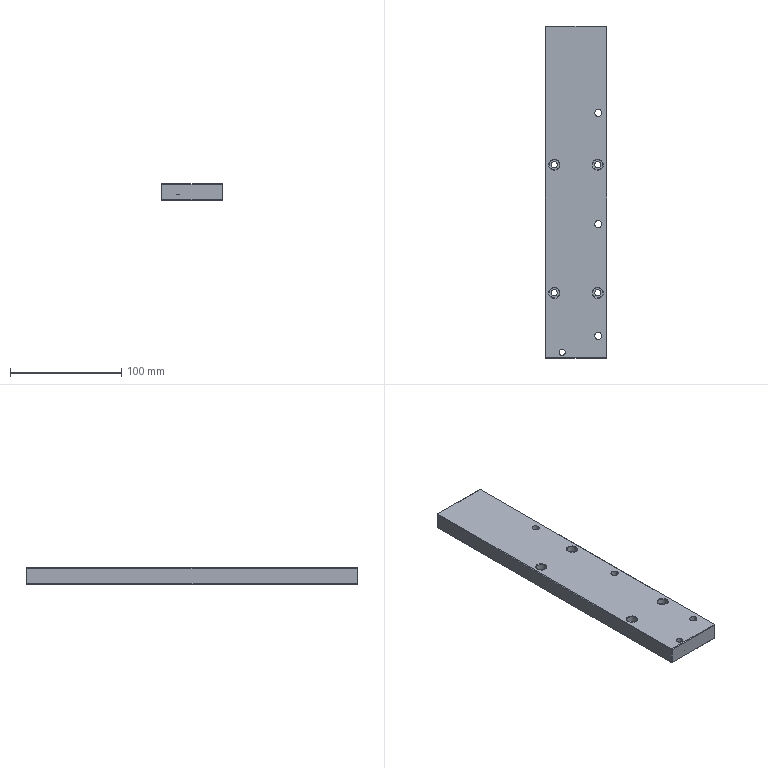Part | 1 solid | 58 faces | box 55 x 298 x 15 mm | volume 240058 mm3 | plane 34 | cylinder 16 | cone 8 | commonest cylinder face diameters 5.5 x5 9 x5 6.5 x3 11 x3
STEP:
#1=CARTESIAN_POINT('',(44.999,-413.,287.5));
#2=VERTEX_POINT('',#1);
#3=CARTESIAN_POINT('',(49.499,-413.,287.5));
#4=DIRECTION('',(0.,0.,-1.));
#5=DIRECTION('',(-1.,0.,0.));
#6=AXIS2_PLACEMENT_3D('',#3,#4,#5);
#7=CIRCLE('',#6,4.5);
#8=EDGE_CURVE('',#2,#2,#7,.T.);
#9=ORIENTED_EDGE('',*,*,#8,.F.);
#10=EDGE_LOOP('',(#9));
#11=FACE_BOUND('',#10,.T.);
#12=CARTESIAN_POINT('',(47.32,-417.5,287.));
#13=VERTEX_POINT('',#12);
#14=CARTESIAN_POINT('',(51.679,-417.5,287.));
#15=VERTEX_POINT('',#14);
#16=CARTESIAN_POINT('',(47.32,-417.5,287.));
#17=CARTESIAN_POINT('',(48.737,-417.825,287.325));
#18=CARTESIAN_POINT('',(50.261,-417.825,287.325));
#19=CARTESIAN_POINT('',(51.679,-417.5,287.));
#20=B_SPLINE_CURVE_WITH_KNOTS('',3,(#16,#17,#18,#19),.UNSPECIFIED.,.F.,.F.,(4,4),(0.,0.004404),.UNSPECIFIED.);
#21=EDGE_CURVE('',#13,#15,#20,.T.);
#22=ORIENTED_EDGE('',*,*,#21,.F.);
#23=CARTESIAN_POINT('',(49.499,-413.,287.));
#24=DIRECTION('',(0.,0.,-1.));
#25=DIRECTION('',(-1.,0.,0.));
#26=AXIS2_PLACEMENT_3D('',#23,#24,#25);
#27=CIRCLE('',#26,5.);
#28=EDGE_CURVE('',#15,#13,#27,.F.);
#29=ORIENTED_EDGE('',*,*,#28,.F.);
#30=EDGE_LOOP('',(#22,#29));
#31=FACE_BOUND('',#30,.T.);
#32=CARTESIAN_POINT('',(49.499,-413.,287.));
#33=DIRECTION('',(0.,0.,-1.));
#34=DIRECTION('',(-1.,0.,0.));
#35=AXIS2_PLACEMENT_3D('',#32,#33,#34);
#36=CONICAL_SURFACE('',#35,5.,0.7854);
#37=ADVANCED_FACE('',(#11,#31),#36,.F.);
#38=CARTESIAN_POINT('',(88.999,-120.,287.5));
#39=VERTEX_POINT('',#38);
#40=CARTESIAN_POINT('',(88.999,-120.5,287.));
#41=VERTEX_POINT('',#40);
#42=CARTESIAN_POINT('',(88.999,-120.5,287.));
#43=DIRECTION('',(0.,-0.7071,-0.7071));
#44=VECTOR('',#43,1000.);
#45=LINE('',#42,#44);
#46=EDGE_CURVE('',#39,#41,#45,.T.);
#47=ORIENTED_EDGE('',*,*,#46,.T.);
#48=CARTESIAN_POINT('',(34.999,-120.5,287.));
#49=VERTEX_POINT('',#48);
#50=CARTESIAN_POINT('',(61.999,-120.5,287.));
#51=DIRECTION('',(1.,0.,0.));
#52=VECTOR('',#51,1000.);
#53=LINE('',#50,#52);
#54=EDGE_CURVE('',#49,#41,#53,.T.);
#55=ORIENTED_EDGE('',*,*,#54,.F.);
#56=CARTESIAN_POINT('',(34.999,-120.,287.5));
#57=VERTEX_POINT('',#56);
#58=CARTESIAN_POINT('',(34.999,-120.,287.5));
#59=DIRECTION('',(0.,0.7071,0.7071));
#60=VECTOR('',#59,1000.);
#61=LINE('',#58,#60);
#62=EDGE_CURVE('',#49,#57,#61,.T.);
#63=ORIENTED_EDGE('',*,*,#62,.T.);
#64=CARTESIAN_POINT('',(38.999,-120.,287.5));
#65=DIRECTION('',(-1.,0.,0.));
#66=VECTOR('',#65,1000.);
#67=LINE('',#64,#66);
#68=EDGE_CURVE('',#39,#57,#67,.T.);
#69=ORIENTED_EDGE('',*,*,#68,.F.);
#70=EDGE_LOOP('',(#47,#55,#63,#69));
#71=FACE_BOUND('',#70,.T.);
#72=CARTESIAN_POINT('',(38.999,-120.,287.5));
#73=DIRECTION('',(0.,0.7071,-0.7071));
#74=DIRECTION('',(1.,0.,0.));
#75=AXIS2_PLACEMENT_3D('',#72,#73,#74);
#76=PLANE('',#75);
#77=ADVANCED_FACE('',(#71),#76,.T.);
#78=CARTESIAN_POINT('',(34.499,-120.5,287.5));
#79=VERTEX_POINT('',#78);
#80=CARTESIAN_POINT('',(34.749,-120.5,287.25));
#81=DIRECTION('',(-0.7071,-0.000000072,0.7071));
#82=VECTOR('',#81,1000.);
#83=LINE('',#80,#82);
#84=EDGE_CURVE('',#49,#79,#83,.T.);
#85=ORIENTED_EDGE('',*,*,#84,.T.);
#86=CARTESIAN_POINT('',(34.999,-120.,287.5));
#87=DIRECTION('',(0.7071,0.7071,0.000000072));
#88=VECTOR('',#87,1000.);
#89=LINE('',#86,#88);
#90=EDGE_CURVE('',#79,#57,#89,.T.);
#91=ORIENTED_EDGE('',*,*,#90,.T.);
#92=ORIENTED_EDGE('',*,*,#62,.F.);
#93=EDGE_LOOP('',(#85,#91,#92));
#94=FACE_BOUND('',#93,.T.);
#95=CARTESIAN_POINT('',(34.999,-120.,287.5));
#96=DIRECTION('',(-0.5774,0.5774,-0.5774));
#97=DIRECTION('',(-0.7071,-0.7071,0.));
#98=AXIS2_PLACEMENT_3D('',#95,#96,#97);
#99=PLANE('',#98);
#100=ADVANCED_FACE('',(#94),#99,.T.);
#101=CARTESIAN_POINT('',(89.499,-120.5,287.5));
#102=VERTEX_POINT('',#101);
#103=CARTESIAN_POINT('',(89.249,-120.25,287.5));
#104=DIRECTION('',(0.7071,-0.7071,-0.000000072));
#105=VECTOR('',#104,1000.);
#106=LINE('',#103,#105);
#107=EDGE_CURVE('',#39,#102,#106,.T.);
#108=ORIENTED_EDGE('',*,*,#107,.T.);
#109=CARTESIAN_POINT('',(88.999,-120.5,287.));
#110=DIRECTION('',(-0.7071,0.000000072,-0.7071));
#111=VECTOR('',#110,1000.);
#112=LINE('',#109,#111);
#113=EDGE_CURVE('',#102,#41,#112,.T.);
#114=ORIENTED_EDGE('',*,*,#113,.T.);
#115=ORIENTED_EDGE('',*,*,#46,.F.);
#116=EDGE_LOOP('',(#108,#114,#115));
#117=FACE_BOUND('',#116,.T.);
#118=CARTESIAN_POINT('',(88.999,-120.5,287.));
#119=DIRECTION('',(0.5774,0.5774,-0.5774));
#120=DIRECTION('',(-0.7071,0.7071,0.));
#121=AXIS2_PLACEMENT_3D('',#118,#119,#120);
#122=PLANE('',#121);
#123=ADVANCED_FACE('',(#117),#122,.T.);
#124=CARTESIAN_POINT('',(34.999,-417.5,287.));
#125=VERTEX_POINT('',#124);
#126=CARTESIAN_POINT('',(34.499,-417.5,287.5));
#127=VERTEX_POINT('',#126);
#128=CARTESIAN_POINT('',(34.499,-417.5,287.5));
#129=DIRECTION('',(-0.7071,-0.000000072,0.7071));
#130=VECTOR('',#129,1000.);
#131=LINE('',#128,#130);
#132=EDGE_CURVE('',#125,#127,#131,.T.);
#133=ORIENTED_EDGE('',*,*,#132,.T.);
#134=CARTESIAN_POINT('',(34.499,-424.5,287.5));
#135=DIRECTION('',(0.,-1.,-0.000000102));
#136=VECTOR('',#135,1000.);
#137=LINE('',#134,#136);
#138=EDGE_CURVE('',#79,#127,#137,.T.);
#139=ORIENTED_EDGE('',*,*,#138,.F.);
#140=ORIENTED_EDGE('',*,*,#84,.F.);
#141=CARTESIAN_POINT('',(34.999,-269.065,287.));
#142=DIRECTION('',(0.000000102,1.,0.));
#143=VECTOR('',#142,1000.);
#144=LINE('',#141,#143);
#145=EDGE_CURVE('',#125,#49,#144,.T.);
#146=ORIENTED_EDGE('',*,*,#145,.F.);
#147=EDGE_LOOP('',(#133,#139,#140,#146));
#148=FACE_BOUND('',#147,.T.);
#149=CARTESIAN_POINT('',(34.499,-424.5,287.5));
#150=DIRECTION('',(-0.7071,0.000000072,-0.7071));
#151=DIRECTION('',(0.,1.,0.000000102));
#152=AXIS2_PLACEMENT_3D('',#149,#150,#151);
#153=PLANE('',#152);
#154=ADVANCED_FACE('',(#148),#153,.T.);
#155=CARTESIAN_POINT('',(34.499,-120.5,301.5));
#156=VERTEX_POINT('',#155);
#157=CARTESIAN_POINT('',(34.999,-120.,301.5));
#158=VERTEX_POINT('',#157);
#159=CARTESIAN_POINT('',(34.499,-120.5,301.5));
#160=DIRECTION('',(0.7071,0.7071,0.000000072));
#161=VECTOR('',#160,1000.);
#162=LINE('',#159,#161);
#163=EDGE_CURVE('',#156,#158,#162,.T.);
#164=ORIENTED_EDGE('',*,*,#163,.T.);
#165=CARTESIAN_POINT('',(34.999,-120.,305.));
#166=DIRECTION('',(0.,-0.000000102,1.));
#167=VECTOR('',#166,1000.);
#168=LINE('',#165,#167);
#169=EDGE_CURVE('',#57,#158,#168,.T.);
#170=ORIENTED_EDGE('',*,*,#169,.F.);
#171=ORIENTED_EDGE('',*,*,#90,.F.);
#172=CARTESIAN_POINT('',(34.499,-120.5,246.881));
#173=DIRECTION('',(0.,0.000000102,-1.));
#174=VECTOR('',#173,1000.);
#175=LINE('',#172,#174);
#176=EDGE_CURVE('',#156,#79,#175,.T.);
#177=ORIENTED_EDGE('',*,*,#176,.F.);
#178=EDGE_LOOP('',(#164,#170,#171,#177));
#179=FACE_BOUND('',#178,.T.);
#180=CARTESIAN_POINT('',(34.999,-120.,305.));
#181=DIRECTION('',(0.7071,-0.7071,-0.000000072));
#182=DIRECTION('',(0.,-0.000000102,1.));
#183=AXIS2_PLACEMENT_3D('',#180,#181,#182);
#184=PLANE('',#183);
#185=ADVANCED_FACE('',(#179),#184,.F.);
#186=CARTESIAN_POINT('',(88.999,-120.,301.5));
#187=VERTEX_POINT('',#186);
#188=CARTESIAN_POINT('',(89.499,-120.5,301.5));
#189=VERTEX_POINT('',#188);
#190=CARTESIAN_POINT('',(89.249,-120.25,301.5));
#191=DIRECTION('',(0.7071,-0.7071,-0.000000072));
#192=VECTOR('',#191,1000.);
#193=LINE('',#190,#192);
#194=EDGE_CURVE('',#187,#189,#193,.T.);
#195=ORIENTED_EDGE('',*,*,#194,.T.);
#196=CARTESIAN_POINT('',(89.499,-120.5,288.5));
#197=DIRECTION('',(0.,-0.000000102,1.));
#198=VECTOR('',#197,1000.);
#199=LINE('',#196,#198);
#200=EDGE_CURVE('',#102,#189,#199,.T.);
#201=ORIENTED_EDGE('',*,*,#200,.F.);
#202=ORIENTED_EDGE('',*,*,#107,.F.);
#203=CARTESIAN_POINT('',(88.999,-120.,305.));
#204=DIRECTION('',(0.,0.000000102,-1.));
#205=VECTOR('',#204,1000.);
#206=LINE('',#203,#205);
#207=EDGE_CURVE('',#187,#39,#206,.T.);
#208=ORIENTED_EDGE('',*,*,#207,.F.);
#209=EDGE_LOOP('',(#195,#201,#202,#208));
#210=FACE_BOUND('',#209,.T.);
#211=CARTESIAN_POINT('',(89.499,-120.5,288.5));
#212=DIRECTION('',(0.7071,0.7071,0.000000072));
#213=DIRECTION('',(0.,0.000000102,-1.));
#214=AXIS2_PLACEMENT_3D('',#211,#212,#213);
#215=PLANE('',#214);
#216=ADVANCED_FACE('',(#210),#215,.T.);
#217=CARTESIAN_POINT('',(89.499,-417.5,287.5));
#218=VERTEX_POINT('',#217);
#219=CARTESIAN_POINT('',(88.999,-417.5,287.));
#220=VERTEX_POINT('',#219);
#221=CARTESIAN_POINT('',(88.999,-417.5,287.));
#222=DIRECTION('',(-0.7071,0.000000072,-0.7071));
#223=VECTOR('',#222,1000.);
#224=LINE('',#221,#223);
#225=EDGE_CURVE('',#218,#220,#224,.T.);
#226=ORIENTED_EDGE('',*,*,#225,.T.);
#227=CARTESIAN_POINT('',(88.999,-248.,287.));
#228=DIRECTION('',(0.000000102,-1.,0.));
#229=VECTOR('',#228,1000.);
#230=LINE('',#227,#229);
#231=EDGE_CURVE('',#41,#220,#230,.T.);
#232=ORIENTED_EDGE('',*,*,#231,.F.);
#233=ORIENTED_EDGE('',*,*,#113,.F.);
#234=CARTESIAN_POINT('',(89.499,-248.,287.5));
#235=DIRECTION('',(0.,1.,0.000000102));
#236=VECTOR('',#235,1000.);
#237=LINE('',#234,#236);
#238=EDGE_CURVE('',#218,#102,#237,.T.);
#239=ORIENTED_EDGE('',*,*,#238,.F.);
#240=EDGE_LOOP('',(#226,#232,#233,#239));
#241=FACE_BOUND('',#240,.T.);
#242=CARTESIAN_POINT('',(89.499,-248.,287.5));
#243=DIRECTION('',(-0.7071,-0.000000072,0.7071));
#244=DIRECTION('',(0.,1.,0.000000102));
#245=AXIS2_PLACEMENT_3D('',#242,#243,#244);
#246=PLANE('',#245);
#247=ADVANCED_FACE('',(#241),#246,.F.);
#248=CARTESIAN_POINT('',(34.999,-418.,287.5));
#249=VERTEX_POINT('',#248);
#250=CARTESIAN_POINT('',(34.999,-417.75,287.25));
#251=DIRECTION('',(0.,-0.7071,0.7071));
#252=VECTOR('',#251,1000.);
#253=LINE('',#250,#252);
#254=EDGE_CURVE('',#125,#249,#253,.T.);
#255=ORIENTED_EDGE('',*,*,#254,.T.);
#256=CARTESIAN_POINT('',(34.499,-417.5,287.5));
#257=DIRECTION('',(-0.7071,0.7071,0.000000072));
#258=VECTOR('',#257,1000.);
#259=LINE('',#256,#258);
#260=EDGE_CURVE('',#249,#127,#259,.T.);
#261=ORIENTED_EDGE('',*,*,#260,.T.);
#262=ORIENTED_EDGE('',*,*,#132,.F.);
#263=EDGE_LOOP('',(#255,#261,#262));
#264=FACE_BOUND('',#263,.T.);
#265=CARTESIAN_POINT('',(34.499,-417.5,287.5));
#266=DIRECTION('',(-0.5774,-0.5774,-0.5774));
#267=DIRECTION('',(-0.7071,0.,0.7071));
#268=AXIS2_PLACEMENT_3D('',#265,#266,#267);
#269=PLANE('',#268);
#270=ADVANCED_FACE('',(#264),#269,.T.);
#271=CARTESIAN_POINT('',(34.999,-120.5,302.));
#272=VERTEX_POINT('',#271);
#273=CARTESIAN_POINT('',(34.499,-120.5,301.5));
#274=DIRECTION('',(0.7071,-0.000000072,0.7071));
#275=VECTOR('',#274,1000.);
#276=LINE('',#273,#275);
#277=EDGE_CURVE('',#156,#272,#276,.T.);
#278=ORIENTED_EDGE('',*,*,#277,.T.);
#279=CARTESIAN_POINT('',(34.999,-120.25,301.75));
#280=DIRECTION('',(0.,0.7071,-0.7071));
#281=VECTOR('',#280,1000.);
#282=LINE('',#279,#281);
#283=EDGE_CURVE('',#272,#158,#282,.T.);
#284=ORIENTED_EDGE('',*,*,#283,.T.);
#285=ORIENTED_EDGE('',*,*,#163,.F.);
#286=EDGE_LOOP('',(#278,#284,#285));
#287=FACE_BOUND('',#286,.T.);
#288=CARTESIAN_POINT('',(34.499,-120.5,301.5));
#289=DIRECTION('',(-0.5774,0.5774,0.5774));
#290=DIRECTION('',(0.7071,0.,0.7071));
#291=AXIS2_PLACEMENT_3D('',#288,#289,#290);
#292=PLANE('',#291);
#293=ADVANCED_FACE('',(#287),#292,.T.);
#294=CARTESIAN_POINT('',(88.999,-120.5,302.));
#295=VERTEX_POINT('',#294);
#296=CARTESIAN_POINT('',(88.999,-120.5,302.));
#297=DIRECTION('',(0.,-0.7071,0.7071));
#298=VECTOR('',#297,1000.);
#299=LINE('',#296,#298);
#300=EDGE_CURVE('',#187,#295,#299,.T.);
#301=ORIENTED_EDGE('',*,*,#300,.T.);
#302=CARTESIAN_POINT('',(88.999,-120.5,302.));
#303=DIRECTION('',(0.7071,0.000000072,-0.7071));
#304=VECTOR('',#303,1000.);
#305=LINE('',#302,#304);
#306=EDGE_CURVE('',#295,#189,#305,.T.);
#307=ORIENTED_EDGE('',*,*,#306,.T.);
#308=ORIENTED_EDGE('',*,*,#194,.F.);
#309=EDGE_LOOP('',(#301,#307,#308));
#310=FACE_BOUND('',#309,.T.);
#311=CARTESIAN_POINT('',(88.999,-120.5,302.));
#312=DIRECTION('',(0.5774,0.5774,0.5774));
#313=DIRECTION('',(0.7071,0.,-0.7071));
#314=AXIS2_PLACEMENT_3D('',#311,#312,#313);
#315=PLANE('',#314);
#316=ADVANCED_FACE('',(#310),#315,.T.);
#317=CARTESIAN_POINT('',(88.999,-418.,287.5));
#318=VERTEX_POINT('',#317);
#319=CARTESIAN_POINT('',(89.249,-417.75,287.5));
#320=DIRECTION('',(-0.7071,-0.7071,-0.000000072));
#321=VECTOR('',#320,1000.);
#322=LINE('',#319,#321);
#323=EDGE_CURVE('',#218,#318,#322,.T.);
#324=ORIENTED_EDGE('',*,*,#323,.T.);
#325=CARTESIAN_POINT('',(88.999,-417.5,287.));
#326=DIRECTION('',(0.,0.7071,-0.7071));
#327=VECTOR('',#326,1000.);
#328=LINE('',#325,#327);
#329=EDGE_CURVE('',#318,#220,#328,.T.);
#330=ORIENTED_EDGE('',*,*,#329,.T.);
#331=ORIENTED_EDGE('',*,*,#225,.F.);
#332=EDGE_LOOP('',(#324,#330,#331));
#333=FACE_BOUND('',#332,.T.);
#334=CARTESIAN_POINT('',(88.999,-417.5,287.));
#335=DIRECTION('',(0.5774,-0.5774,-0.5774));
#336=DIRECTION('',(-0.7071,0.,-0.7071));
#337=AXIS2_PLACEMENT_3D('',#334,#335,#336);
#338=PLANE('',#337);
#339=ADVANCED_FACE('',(#333),#338,.T.);
#340=CARTESIAN_POINT('',(35.999,-417.5,287.));
#341=DIRECTION('',(-1.,0.,0.));
#342=VECTOR('',#341,1000.);
#343=LINE('',#340,#342);
#344=EDGE_CURVE('',#13,#125,#343,.T.);
#345=ORIENTED_EDGE('',*,*,#344,.F.);
#346=ORIENTED_EDGE('',*,*,#21,.T.);
#347=CARTESIAN_POINT('',(35.999,-417.5,287.));
#348=DIRECTION('',(-1.,0.,0.));
#349=VECTOR('',#348,1000.);
#350=LINE('',#347,#349);
#351=EDGE_CURVE('',#220,#15,#350,.T.);
#352=ORIENTED_EDGE('',*,*,#351,.F.);
#353=ORIENTED_EDGE('',*,*,#329,.F.);
#354=CARTESIAN_POINT('',(35.999,-418.,287.5));
#355=DIRECTION('',(1.,0.,0.));
#356=VECTOR('',#355,1000.);
#357=LINE('',#354,#356);
#358=EDGE_CURVE('',#249,#318,#357,.T.);
#359=ORIENTED_EDGE('',*,*,#358,.F.);
#360=ORIENTED_EDGE('',*,*,#254,.F.);
#361=EDGE_LOOP('',(#345,#346,#352,#353,#359,#360));
#362=FACE_BOUND('',#361,.T.);
#363=CARTESIAN_POINT('',(35.999,-418.,287.5));
#364=DIRECTION('',(0.,0.7071,0.7071));
#365=DIRECTION('',(1.,0.,0.));
#366=AXIS2_PLACEMENT_3D('',#363,#364,#365);
#367=PLANE('',#366);
#368=ADVANCED_FACE('',(#362),#367,.F.);
#369=CARTESIAN_POINT('',(34.999,-418.,301.5));
#370=VERTEX_POINT('',#369);
#371=CARTESIAN_POINT('',(34.499,-417.5,301.5));
#372=VERTEX_POINT('',#371);
#373=CARTESIAN_POINT('',(34.999,-418.,301.5));
#374=DIRECTION('',(-0.7071,0.7071,0.000000072));
#375=VECTOR('',#374,1000.);
#376=LINE('',#373,#375);
#377=EDGE_CURVE('',#370,#372,#376,.T.);
#378=ORIENTED_EDGE('',*,*,#377,.T.);
#379=CARTESIAN_POINT('',(34.499,-417.5,246.881));
#380=DIRECTION('',(0.,-0.000000102,1.));
#381=VECTOR('',#380,1000.);
#382=LINE('',#379,#381);
#383=EDGE_CURVE('',#127,#372,#382,.T.);
#384=ORIENTED_EDGE('',*,*,#383,.F.);
#385=ORIENTED_EDGE('',*,*,#260,.F.);
#386=CARTESIAN_POINT('',(34.999,-418.,314.323));
#387=DIRECTION('',(0.,0.000000102,-1.));
#388=VECTOR('',#387,1000.);
#389=LINE('',#386,#388);
#390=EDGE_CURVE('',#370,#249,#389,.T.);
#391=ORIENTED_EDGE('',*,*,#390,.F.);
#392=EDGE_LOOP('',(#378,#384,#385,#391));
#393=FACE_BOUND('',#392,.T.);
#394=CARTESIAN_POINT('',(34.499,-417.5,246.881));
#395=DIRECTION('',(-0.7071,-0.7071,-0.000000072));
#396=DIRECTION('',(0.,0.000000102,-1.));
#397=AXIS2_PLACEMENT_3D('',#394,#395,#396);
#398=PLANE('',#397);
#399=ADVANCED_FACE('',(#393),#398,.T.);
#400=CARTESIAN_POINT('',(34.999,-417.5,302.));
#401=VERTEX_POINT('',#400);
#402=CARTESIAN_POINT('',(34.749,-417.5,301.75));
#403=DIRECTION('',(0.7071,-0.000000072,0.7071));
#404=VECTOR('',#403,1000.);
#405=LINE('',#402,#404);
#406=EDGE_CURVE('',#372,#401,#405,.T.);
#407=ORIENTED_EDGE('',*,*,#406,.T.);
#408=CARTESIAN_POINT('',(34.999,-269.,302.));
#409=DIRECTION('',(0.000000102,-1.,0.));
#410=VECTOR('',#409,1000.);
#411=LINE('',#408,#410);
#412=EDGE_CURVE('',#272,#401,#411,.T.);
#413=ORIENTED_EDGE('',*,*,#412,.F.);
#414=ORIENTED_EDGE('',*,*,#277,.F.);
#415=CARTESIAN_POINT('',(34.499,-120.,301.5));
#416=DIRECTION('',(0.,1.,0.000000102));
#417=VECTOR('',#416,1000.);
#418=LINE('',#415,#417);
#419=EDGE_CURVE('',#372,#156,#418,.T.);
#420=ORIENTED_EDGE('',*,*,#419,.F.);
#421=EDGE_LOOP('',(#407,#413,#414,#420));
#422=FACE_BOUND('',#421,.T.);
#423=CARTESIAN_POINT('',(34.999,-249.,302.));
#424=DIRECTION('',(0.7071,0.000000072,-0.7071));
#425=DIRECTION('',(0.,-1.,-0.000000102));
#426=AXIS2_PLACEMENT_3D('',#423,#424,#425);
#427=PLANE('',#426);
#428=ADVANCED_FACE('',(#422),#427,.F.);
#429=ORIENTED_EDGE('',*,*,#283,.F.);
#430=CARTESIAN_POINT('',(61.999,-120.5,302.));
#431=DIRECTION('',(-1.,0.,0.));
#432=VECTOR('',#431,1000.);
#433=LINE('',#430,#432);
#434=EDGE_CURVE('',#295,#272,#433,.T.);
#435=ORIENTED_EDGE('',*,*,#434,.F.);
#436=ORIENTED_EDGE('',*,*,#300,.F.);
#437=CARTESIAN_POINT('',(89.499,-120.,301.5));
#438=DIRECTION('',(1.,0.,0.));
#439=VECTOR('',#438,1000.);
#440=LINE('',#437,#439);
#441=EDGE_CURVE('',#158,#187,#440,.T.);
#442=ORIENTED_EDGE('',*,*,#441,.F.);
#443=EDGE_LOOP('',(#429,#435,#436,#442));
#444=FACE_BOUND('',#443,.T.);
#445=CARTESIAN_POINT('',(81.999,-120.5,302.));
#446=DIRECTION('',(0.,-0.7071,-0.7071));
#447=DIRECTION('',(-1.,0.,0.));
#448=AXIS2_PLACEMENT_3D('',#445,#446,#447);
#449=PLANE('',#448);
#450=ADVANCED_FACE('',(#444),#449,.F.);
#451=CARTESIAN_POINT('',(88.999,-417.5,302.));
#452=VERTEX_POINT('',#451);
#453=CARTESIAN_POINT('',(89.499,-417.5,301.5));
#454=VERTEX_POINT('',#453);
#455=CARTESIAN_POINT('',(89.249,-417.5,301.75));
#456=DIRECTION('',(0.7071,0.000000072,-0.7071));
#457=VECTOR('',#456,1000.);
#458=LINE('',#455,#457);
#459=EDGE_CURVE('',#452,#454,#458,.T.);
#460=ORIENTED_EDGE('',*,*,#459,.T.);
#461=CARTESIAN_POINT('',(89.499,-418.,301.5));
#462=DIRECTION('',(0.,-1.,-0.000000102));
#463=VECTOR('',#462,1000.);
#464=LINE('',#461,#463);
#465=EDGE_CURVE('',#189,#454,#464,.T.);
#466=ORIENTED_EDGE('',*,*,#465,.F.);
#467=ORIENTED_EDGE('',*,*,#306,.F.);
#468=CARTESIAN_POINT('',(88.999,-249.,302.));
#469=DIRECTION('',(0.000000102,1.,0.));
#470=VECTOR('',#469,1000.);
#471=LINE('',#468,#470);
#472=EDGE_CURVE('',#452,#295,#471,.T.);
#473=ORIENTED_EDGE('',*,*,#472,.F.);
#474=EDGE_LOOP('',(#460,#466,#467,#473));
#475=FACE_BOUND('',#474,.T.);
#476=CARTESIAN_POINT('',(88.999,-249.,302.));
#477=DIRECTION('',(0.7071,-0.000000072,0.7071));
#478=DIRECTION('',(0.,-1.,-0.000000102));
#479=AXIS2_PLACEMENT_3D('',#476,#477,#478);
#480=PLANE('',#479);
#481=ADVANCED_FACE('',(#475),#480,.T.);
#482=CARTESIAN_POINT('',(88.999,-418.,301.5));
#483=VERTEX_POINT('',#482);
#484=CARTESIAN_POINT('',(88.999,-418.,301.5));
#485=DIRECTION('',(-0.7071,-0.7071,-0.000000072));
#486=VECTOR('',#485,1000.);
#487=LINE('',#484,#486);
#488=EDGE_CURVE('',#454,#483,#487,.T.);
#489=ORIENTED_EDGE('',*,*,#488,.T.);
#490=CARTESIAN_POINT('',(88.999,-418.,314.323));
#491=DIRECTION('',(0.,-0.000000102,1.));
#492=VECTOR('',#491,1000.);
#493=LINE('',#490,#492);
#494=EDGE_CURVE('',#318,#483,#493,.T.);
#495=ORIENTED_EDGE('',*,*,#494,.F.);
#496=ORIENTED_EDGE('',*,*,#323,.F.);
#497=CARTESIAN_POINT('',(89.499,-417.5,288.5));
#498=DIRECTION('',(0.,0.000000102,-1.));
#499=VECTOR('',#498,1000.);
#500=LINE('',#497,#499);
#501=EDGE_CURVE('',#454,#218,#500,.T.);
#502=ORIENTED_EDGE('',*,*,#501,.F.);
#503=EDGE_LOOP('',(#489,#495,#496,#502));
#504=FACE_BOUND('',#503,.T.);
#505=CARTESIAN_POINT('',(88.999,-418.,314.323));
#506=DIRECTION('',(-0.7071,0.7071,0.000000072));
#507=DIRECTION('',(0.,-0.000000102,1.));
#508=AXIS2_PLACEMENT_3D('',#505,#506,#507);
#509=PLANE('',#508);
#510=ADVANCED_FACE('',(#504),#509,.F.);
#511=ORIENTED_EDGE('',*,*,#377,.F.);
#512=CARTESIAN_POINT('',(34.999,-418.,301.5));
#513=DIRECTION('',(0.,0.7071,0.7071));
#514=VECTOR('',#513,1000.);
#515=LINE('',#512,#514);
#516=EDGE_CURVE('',#370,#401,#515,.T.);
#517=ORIENTED_EDGE('',*,*,#516,.T.);
#518=ORIENTED_EDGE('',*,*,#406,.F.);
#519=EDGE_LOOP('',(#511,#517,#518));
#520=FACE_BOUND('',#519,.T.);
#521=CARTESIAN_POINT('',(34.999,-418.,301.5));
#522=DIRECTION('',(-0.5774,-0.5774,0.5774));
#523=DIRECTION('',(0.7071,-0.7071,0.));
#524=AXIS2_PLACEMENT_3D('',#521,#522,#523);
#525=PLANE('',#524);
#526=ADVANCED_FACE('',(#520),#525,.T.);
#527=ORIENTED_EDGE('',*,*,#459,.F.);
#528=CARTESIAN_POINT('',(88.999,-418.,301.5));
#529=DIRECTION('',(0.,-0.7071,-0.7071));
#530=VECTOR('',#529,1000.);
#531=LINE('',#528,#530);
#532=EDGE_CURVE('',#452,#483,#531,.T.);
#533=ORIENTED_EDGE('',*,*,#532,.T.);
#534=ORIENTED_EDGE('',*,*,#488,.F.);
#535=EDGE_LOOP('',(#527,#533,#534));
#536=FACE_BOUND('',#535,.T.);
#537=CARTESIAN_POINT('',(88.999,-418.,301.5));
#538=DIRECTION('',(0.5774,-0.5774,0.5774));
#539=DIRECTION('',(0.7071,0.7071,0.));
#540=AXIS2_PLACEMENT_3D('',#537,#538,#539);
#541=PLANE('',#540);
#542=ADVANCED_FACE('',(#536),#541,.T.);
#543=ORIENTED_EDGE('',*,*,#532,.F.);
#544=CARTESIAN_POINT('',(81.999,-417.5,302.));
#545=DIRECTION('',(1.,0.,0.));
#546=VECTOR('',#545,1000.);
#547=LINE('',#544,#546);
#548=EDGE_CURVE('',#401,#452,#547,.T.);
#549=ORIENTED_EDGE('',*,*,#548,.F.);
#550=ORIENTED_EDGE('',*,*,#516,.F.);
#551=CARTESIAN_POINT('',(34.499,-418.,301.5));
#552=DIRECTION('',(-1.,0.,0.));
#553=VECTOR('',#552,1000.);
#554=LINE('',#551,#553);
#555=EDGE_CURVE('',#483,#370,#554,.T.);
#556=ORIENTED_EDGE('',*,*,#555,.F.);
#557=EDGE_LOOP('',(#543,#549,#550,#556));
#558=FACE_BOUND('',#557,.T.);
#559=CARTESIAN_POINT('',(81.999,-417.5,302.));
#560=DIRECTION('',(0.,-0.7071,0.7071));
#561=DIRECTION('',(-1.,0.,0.));
#562=AXIS2_PLACEMENT_3D('',#559,#560,#561);
#563=PLANE('',#562);
#564=ADVANCED_FACE('',(#558),#563,.T.);
#565=CARTESIAN_POINT('',(76.499,-198.,287.5));
#566=VERTEX_POINT('',#565);
#567=CARTESIAN_POINT('',(81.999,-198.,287.5));
#568=DIRECTION('',(0.,0.,-1.));
#569=DIRECTION('',(-1.,0.,0.));
#570=AXIS2_PLACEMENT_3D('',#567,#568,#569);
#571=CIRCLE('',#570,5.5);
#572=EDGE_CURVE('',#566,#566,#571,.T.);
#573=ORIENTED_EDGE('',*,*,#572,.F.);
#574=EDGE_LOOP('',(#573));
#575=FACE_BOUND('',#574,.T.);
#576=CARTESIAN_POINT('',(75.999,-198.,287.));
#577=VERTEX_POINT('',#576);
#578=CARTESIAN_POINT('',(81.999,-198.,287.));
#579=DIRECTION('',(0.,0.,1.));
#580=DIRECTION('',(-1.,0.,0.));
#581=AXIS2_PLACEMENT_3D('',#578,#579,#580);
#582=CIRCLE('',#581,6.);
#583=EDGE_CURVE('',#577,#577,#582,.T.);
#584=ORIENTED_EDGE('',*,*,#583,.F.);
#585=EDGE_LOOP('',(#584));
#586=FACE_BOUND('',#585,.T.);
#587=CARTESIAN_POINT('',(81.999,-198.,287.5));
#588=DIRECTION('',(0.,0.,-1.));
#589=DIRECTION('',(-1.,0.,0.));
#590=AXIS2_PLACEMENT_3D('',#587,#588,#589);
#591=CONICAL_SURFACE('',#590,5.5,0.7854);
#592=ADVANCED_FACE('',(#575,#586),#591,.F.);
#593=CARTESIAN_POINT('',(76.499,-298.,287.5));
#594=VERTEX_POINT('',#593);
#595=CARTESIAN_POINT('',(81.999,-298.,287.5));
#596=DIRECTION('',(0.,0.,-1.));
#597=DIRECTION('',(-1.,0.,0.));
#598=AXIS2_PLACEMENT_3D('',#595,#596,#597);
#599=CIRCLE('',#598,5.5);
#600=EDGE_CURVE('',#594,#594,#599,.T.);
#601=ORIENTED_EDGE('',*,*,#600,.F.);
#602=EDGE_LOOP('',(#601));
#603=FACE_BOUND('',#602,.T.);
#604=CARTESIAN_POINT('',(75.999,-298.,287.));
#605=VERTEX_POINT('',#604);
#606=CARTESIAN_POINT('',(81.999,-298.,287.));
#607=DIRECTION('',(0.,0.,1.));
#608=DIRECTION('',(-1.,0.,0.));
#609=AXIS2_PLACEMENT_3D('',#606,#607,#608);
#610=CIRCLE('',#609,6.);
#611=EDGE_CURVE('',#605,#605,#610,.T.);
#612=ORIENTED_EDGE('',*,*,#611,.F.);
#613=EDGE_LOOP('',(#612));
#614=FACE_BOUND('',#613,.T.);
#615=CARTESIAN_POINT('',(81.999,-298.,287.5));
#616=DIRECTION('',(0.,0.,-1.));
#617=DIRECTION('',(-1.,0.,0.));
#618=AXIS2_PLACEMENT_3D('',#615,#616,#617);
#619=CONICAL_SURFACE('',#618,5.5,0.7854);
#620=ADVANCED_FACE('',(#603,#614),#619,.F.);
#621=CARTESIAN_POINT('',(76.499,-398.,287.5));
#622=VERTEX_POINT('',#621);
#623=CARTESIAN_POINT('',(81.999,-398.,287.5));
#624=DIRECTION('',(0.,0.,-1.));
#625=DIRECTION('',(-1.,0.,0.));
#626=AXIS2_PLACEMENT_3D('',#623,#624,#625);
#627=CIRCLE('',#626,5.5);
#628=EDGE_CURVE('',#622,#622,#627,.T.);
#629=ORIENTED_EDGE('',*,*,#628,.F.);
#630=EDGE_LOOP('',(#629));
#631=FACE_BOUND('',#630,.T.);
#632=CARTESIAN_POINT('',(75.999,-398.,287.));
#633=VERTEX_POINT('',#632);
#634=CARTESIAN_POINT('',(81.999,-398.,287.));
#635=DIRECTION('',(0.,0.,-1.));
#636=DIRECTION('',(-1.,0.,0.));
#637=AXIS2_PLACEMENT_3D('',#634,#635,#636);
#638=CIRCLE('',#637,6.);
#639=EDGE_CURVE('',#633,#633,#638,.F.);
#640=ORIENTED_EDGE('',*,*,#639,.F.);
#641=EDGE_LOOP('',(#640));
#642=FACE_BOUND('',#641,.T.);
#643=CARTESIAN_POINT('',(81.999,-398.,287.5));
#644=DIRECTION('',(0.,0.,-1.));
#645=DIRECTION('',(-1.,0.,0.));
#646=AXIS2_PLACEMENT_3D('',#643,#644,#645);
#647=CONICAL_SURFACE('',#646,5.5,0.7854);
#648=ADVANCED_FACE('',(#631,#642),#647,.F.);
#649=CARTESIAN_POINT('',(53.999,-413.,292.5));
#650=VERTEX_POINT('',#649);
#651=CARTESIAN_POINT('',(49.499,-413.,292.5));
#652=DIRECTION('',(0.,0.,1.));
#653=DIRECTION('',(1.,0.,0.));
#654=AXIS2_PLACEMENT_3D('',#651,#652,#653);
#655=CIRCLE('',#654,4.5);
#656=EDGE_CURVE('',#650,#650,#655,.T.);
#657=ORIENTED_EDGE('',*,*,#656,.T.);
#658=EDGE_LOOP('',(#657));
#659=FACE_BOUND('',#658,.T.);
#660=ORIENTED_EDGE('',*,*,#8,.T.);
#661=EDGE_LOOP('',(#660));
#662=FACE_BOUND('',#661,.T.);
#663=CARTESIAN_POINT('',(49.499,-413.,287.));
#664=DIRECTION('',(0.,0.,1.));
#665=DIRECTION('',(1.,0.,0.));
#666=AXIS2_PLACEMENT_3D('',#663,#664,#665);
#667=CYLINDRICAL_SURFACE('',#666,4.5);
#668=ADVANCED_FACE('',(#659,#662),#667,.F.);
#669=CARTESIAN_POINT('',(52.249,-413.,292.5));
#670=VERTEX_POINT('',#669);
#671=CARTESIAN_POINT('',(49.499,-413.,292.5));
#672=DIRECTION('',(0.,0.,-1.));
#673=DIRECTION('',(1.,0.,0.));
#674=AXIS2_PLACEMENT_3D('',#671,#672,#673);
#675=CIRCLE('',#674,2.75);
#676=EDGE_CURVE('',#670,#670,#675,.T.);
#677=ORIENTED_EDGE('',*,*,#676,.F.);
#678=EDGE_LOOP('',(#677));
#679=FACE_BOUND('',#678,.T.);
#680=ORIENTED_EDGE('',*,*,#656,.F.);
#681=EDGE_LOOP('',(#680));
#682=FACE_BOUND('',#681,.T.);
#683=CARTESIAN_POINT('',(49.499,-413.,292.5));
#684=DIRECTION('',(0.,0.,1.));
#685=DIRECTION('',(1.,0.,0.));
#686=AXIS2_PLACEMENT_3D('',#683,#684,#685);
#687=PLANE('',#686);
#688=ADVANCED_FACE('',(#679,#682),#687,.F.);
#689=CARTESIAN_POINT('',(46.749,-413.,302.));
#690=VERTEX_POINT('',#689);
#691=CARTESIAN_POINT('',(49.499,-413.,302.));
#692=DIRECTION('',(0.,0.,-1.));
#693=DIRECTION('',(-1.,0.,0.));
#694=AXIS2_PLACEMENT_3D('',#691,#692,#693);
#695=CIRCLE('',#694,2.75);
#696=EDGE_CURVE('',#690,#690,#695,.T.);
#697=ORIENTED_EDGE('',*,*,#696,.F.);
#698=EDGE_LOOP('',(#697));
#699=FACE_BOUND('',#698,.T.);
#700=ORIENTED_EDGE('',*,*,#676,.T.);
#701=EDGE_LOOP('',(#700));
#702=FACE_BOUND('',#701,.T.);
#703=CARTESIAN_POINT('',(49.499,-413.,302.));
#704=DIRECTION('',(0.,0.,-1.));
#705=DIRECTION('',(1.,0.,0.));
#706=AXIS2_PLACEMENT_3D('',#703,#704,#705);
#707=CYLINDRICAL_SURFACE('',#706,2.75);
#708=ADVANCED_FACE('',(#699,#702),#707,.F.);
#709=CARTESIAN_POINT('',(76.499,-244.5,302.));
#710=VERTEX_POINT('',#709);
#711=CARTESIAN_POINT('',(81.499,-244.5,302.));
#712=DIRECTION('',(0.,0.,-1.));
#713=DIRECTION('',(-1.,0.,0.));
#714=AXIS2_PLACEMENT_3D('',#711,#712,#713);
#715=CIRCLE('',#714,5.);
#716=EDGE_CURVE('',#710,#710,#715,.T.);
#717=ORIENTED_EDGE('',*,*,#716,.F.);
#718=EDGE_LOOP('',(#717));
#719=FACE_BOUND('',#718,.T.);
#720=CARTESIAN_POINT('',(76.999,-244.5,301.5));
#721=VERTEX_POINT('',#720);
#722=CARTESIAN_POINT('',(81.499,-244.5,301.5));
#723=DIRECTION('',(0.,0.,1.));
#724=DIRECTION('',(-1.,0.,0.));
#725=AXIS2_PLACEMENT_3D('',#722,#723,#724);
#726=CIRCLE('',#725,4.5);
#727=EDGE_CURVE('',#721,#721,#726,.T.);
#728=ORIENTED_EDGE('',*,*,#727,.F.);
#729=EDGE_LOOP('',(#728));
#730=FACE_BOUND('',#729,.T.);
#731=CARTESIAN_POINT('',(81.499,-244.5,302.));
#732=DIRECTION('',(0.,0.,1.));
#733=DIRECTION('',(1.,0.,0.));
#734=AXIS2_PLACEMENT_3D('',#731,#732,#733);
#735=CONICAL_SURFACE('',#734,5.,0.7854);
#736=ADVANCED_FACE('',(#719,#730),#735,.F.);
#737=CARTESIAN_POINT('',(37.499,-244.5,302.));
#738=VERTEX_POINT('',#737);
#739=CARTESIAN_POINT('',(42.499,-244.5,302.));
#740=DIRECTION('',(0.,0.,-1.));
#741=DIRECTION('',(-1.,0.,0.));
#742=AXIS2_PLACEMENT_3D('',#739,#740,#741);
#743=CIRCLE('',#742,5.);
#744=EDGE_CURVE('',#738,#738,#743,.T.);
#745=ORIENTED_EDGE('',*,*,#744,.F.);
#746=EDGE_LOOP('',(#745));
#747=FACE_BOUND('',#746,.T.);
#748=CARTESIAN_POINT('',(37.999,-244.5,301.5));
#749=VERTEX_POINT('',#748);
#750=CARTESIAN_POINT('',(42.499,-244.5,301.5));
#751=DIRECTION('',(0.,0.,1.));
#752=DIRECTION('',(-1.,0.,0.));
#753=AXIS2_PLACEMENT_3D('',#750,#751,#752);
#754=CIRCLE('',#753,4.5);
#755=EDGE_CURVE('',#749,#749,#754,.T.);
#756=ORIENTED_EDGE('',*,*,#755,.F.);
#757=EDGE_LOOP('',(#756));
#758=FACE_BOUND('',#757,.T.);
#759=CARTESIAN_POINT('',(42.499,-244.5,302.));
#760=DIRECTION('',(0.,0.,1.));
#761=DIRECTION('',(1.,0.,0.));
#762=AXIS2_PLACEMENT_3D('',#759,#760,#761);
#763=CONICAL_SURFACE('',#762,5.,0.7854);
#764=ADVANCED_FACE('',(#747,#758),#763,.F.);
#765=CARTESIAN_POINT('',(76.499,-359.5,302.));
#766=VERTEX_POINT('',#765);
#767=CARTESIAN_POINT('',(81.499,-359.5,302.));
#768=DIRECTION('',(0.,0.,-1.));
#769=DIRECTION('',(-1.,0.,0.));
#770=AXIS2_PLACEMENT_3D('',#767,#768,#769);
#771=CIRCLE('',#770,5.);
#772=EDGE_CURVE('',#766,#766,#771,.T.);
#773=ORIENTED_EDGE('',*,*,#772,.F.);
#774=EDGE_LOOP('',(#773));
#775=FACE_BOUND('',#774,.T.);
#776=CARTESIAN_POINT('',(76.999,-359.5,301.5));
#777=VERTEX_POINT('',#776);
#778=CARTESIAN_POINT('',(81.499,-359.5,301.5));
#779=DIRECTION('',(0.,0.,1.));
#780=DIRECTION('',(-1.,0.,0.));
#781=AXIS2_PLACEMENT_3D('',#778,#779,#780);
#782=CIRCLE('',#781,4.5);
#783=EDGE_CURVE('',#777,#777,#782,.T.);
#784=ORIENTED_EDGE('',*,*,#783,.F.);
#785=EDGE_LOOP('',(#784));
#786=FACE_BOUND('',#785,.T.);
#787=CARTESIAN_POINT('',(81.499,-359.5,302.));
#788=DIRECTION('',(0.,0.,1.));
#789=DIRECTION('',(1.,0.,0.));
#790=AXIS2_PLACEMENT_3D('',#787,#788,#789);
#791=CONICAL_SURFACE('',#790,5.,0.7854);
#792=ADVANCED_FACE('',(#775,#786),#791,.F.);
#793=CARTESIAN_POINT('',(37.499,-359.5,302.));
#794=VERTEX_POINT('',#793);
#795=CARTESIAN_POINT('',(42.499,-359.5,302.));
#796=DIRECTION('',(0.,0.,-1.));
#797=DIRECTION('',(-1.,0.,0.));
#798=AXIS2_PLACEMENT_3D('',#795,#796,#797);
#799=CIRCLE('',#798,5.);
#800=EDGE_CURVE('',#794,#794,#799,.T.);
#801=ORIENTED_EDGE('',*,*,#800,.F.);
#802=EDGE_LOOP('',(#801));
#803=FACE_BOUND('',#802,.T.);
#804=CARTESIAN_POINT('',(37.999,-359.5,301.5));
#805=VERTEX_POINT('',#804);
#806=CARTESIAN_POINT('',(42.499,-359.5,301.5));
#807=DIRECTION('',(0.,0.,1.));
#808=DIRECTION('',(-1.,0.,0.));
#809=AXIS2_PLACEMENT_3D('',#806,#807,#808);
#810=CIRCLE('',#809,4.5);
#811=EDGE_CURVE('',#805,#805,#810,.T.);
#812=ORIENTED_EDGE('',*,*,#811,.F.);
#813=EDGE_LOOP('',(#812));
#814=FACE_BOUND('',#813,.T.);
#815=CARTESIAN_POINT('',(42.499,-359.5,302.));
#816=DIRECTION('',(0.,0.,1.));
#817=DIRECTION('',(1.,0.,0.));
#818=AXIS2_PLACEMENT_3D('',#815,#816,#817);
#819=CONICAL_SURFACE('',#818,5.,0.7854);
#820=ADVANCED_FACE('',(#803,#814),#819,.F.);
#821=CARTESIAN_POINT('',(37.999,-244.5,296.5));
#822=VERTEX_POINT('',#821);
#823=CARTESIAN_POINT('',(42.499,-244.5,296.5));
#824=DIRECTION('',(0.,0.,-1.));
#825=DIRECTION('',(-1.,0.,0.));
#826=AXIS2_PLACEMENT_3D('',#823,#824,#825);
#827=CIRCLE('',#826,4.5);
#828=EDGE_CURVE('',#822,#822,#827,.T.);
#829=ORIENTED_EDGE('',*,*,#828,.T.);
#830=EDGE_LOOP('',(#829));
#831=FACE_BOUND('',#830,.T.);
#832=ORIENTED_EDGE('',*,*,#755,.T.);
#833=EDGE_LOOP('',(#832));
#834=FACE_BOUND('',#833,.T.);
#835=CARTESIAN_POINT('',(42.499,-244.5,302.));
#836=DIRECTION('',(0.,0.,-1.));
#837=DIRECTION('',(1.,0.,0.));
#838=AXIS2_PLACEMENT_3D('',#835,#836,#837);
#839=CYLINDRICAL_SURFACE('',#838,4.5);
#840=ADVANCED_FACE('',(#831,#834),#839,.F.);
#841=CARTESIAN_POINT('',(39.749,-244.5,296.5));
#842=VERTEX_POINT('',#841);
#843=CARTESIAN_POINT('',(42.499,-244.5,296.5));
#844=DIRECTION('',(0.,0.,-1.));
#845=DIRECTION('',(-1.,0.,0.));
#846=AXIS2_PLACEMENT_3D('',#843,#844,#845);
#847=CIRCLE('',#846,2.75);
#848=EDGE_CURVE('',#842,#842,#847,.F.);
#849=ORIENTED_EDGE('',*,*,#848,.F.);
#850=EDGE_LOOP('',(#849));
#851=FACE_BOUND('',#850,.T.);
#852=ORIENTED_EDGE('',*,*,#828,.F.);
#853=EDGE_LOOP('',(#852));
#854=FACE_BOUND('',#853,.T.);
#855=CARTESIAN_POINT('',(42.499,-359.5,296.5));
#856=DIRECTION('',(0.,0.,-1.));
#857=DIRECTION('',(-1.,0.,0.));
#858=AXIS2_PLACEMENT_3D('',#855,#856,#857);
#859=PLANE('',#858);
#860=ADVANCED_FACE('',(#851,#854),#859,.F.);
#861=CARTESIAN_POINT('',(76.999,-244.5,296.5));
#862=VERTEX_POINT('',#861);
#863=CARTESIAN_POINT('',(81.499,-244.5,296.5));
#864=DIRECTION('',(0.,0.,-1.));
#865=DIRECTION('',(-1.,0.,0.));
#866=AXIS2_PLACEMENT_3D('',#863,#864,#865);
#867=CIRCLE('',#866,4.5);
#868=EDGE_CURVE('',#862,#862,#867,.T.);
#869=ORIENTED_EDGE('',*,*,#868,.T.);
#870=EDGE_LOOP('',(#869));
#871=FACE_BOUND('',#870,.T.);
#872=ORIENTED_EDGE('',*,*,#727,.T.);
#873=EDGE_LOOP('',(#872));
#874=FACE_BOUND('',#873,.T.);
#875=CARTESIAN_POINT('',(81.499,-244.5,302.));
#876=DIRECTION('',(0.,0.,-1.));
#877=DIRECTION('',(1.,0.,0.));
#878=AXIS2_PLACEMENT_3D('',#875,#876,#877);
#879=CYLINDRICAL_SURFACE('',#878,4.5);
#880=ADVANCED_FACE('',(#871,#874),#879,.F.);
#881=CARTESIAN_POINT('',(78.749,-244.5,296.5));
#882=VERTEX_POINT('',#881);
#883=CARTESIAN_POINT('',(81.499,-244.5,296.5));
#884=DIRECTION('',(0.,0.,-1.));
#885=DIRECTION('',(-1.,0.,0.));
#886=AXIS2_PLACEMENT_3D('',#883,#884,#885);
#887=CIRCLE('',#886,2.75);
#888=EDGE_CURVE('',#882,#882,#887,.F.);
#889=ORIENTED_EDGE('',*,*,#888,.F.);
#890=EDGE_LOOP('',(#889));
#891=FACE_BOUND('',#890,.T.);
#892=ORIENTED_EDGE('',*,*,#868,.F.);
#893=EDGE_LOOP('',(#892));
#894=FACE_BOUND('',#893,.T.);
#895=CARTESIAN_POINT('',(42.499,-359.5,296.5));
#896=DIRECTION('',(0.,0.,-1.));
#897=DIRECTION('',(-1.,0.,0.));
#898=AXIS2_PLACEMENT_3D('',#895,#896,#897);
#899=PLANE('',#898);
#900=ADVANCED_FACE('',(#891,#894),#899,.F.);
#901=CARTESIAN_POINT('',(76.999,-359.5,296.5));
#902=VERTEX_POINT('',#901);
#903=CARTESIAN_POINT('',(81.499,-359.5,296.5));
#904=DIRECTION('',(0.,0.,-1.));
#905=DIRECTION('',(-1.,0.,0.));
#906=AXIS2_PLACEMENT_3D('',#903,#904,#905);
#907=CIRCLE('',#906,4.5);
#908=EDGE_CURVE('',#902,#902,#907,.T.);
#909=ORIENTED_EDGE('',*,*,#908,.T.);
#910=EDGE_LOOP('',(#909));
#911=FACE_BOUND('',#910,.T.);
#912=ORIENTED_EDGE('',*,*,#783,.T.);
#913=EDGE_LOOP('',(#912));
#914=FACE_BOUND('',#913,.T.);
#915=CARTESIAN_POINT('',(81.499,-359.5,302.));
#916=DIRECTION('',(0.,0.,-1.));
#917=DIRECTION('',(1.,0.,0.));
#918=AXIS2_PLACEMENT_3D('',#915,#916,#917);
#919=CYLINDRICAL_SURFACE('',#918,4.5);
#920=ADVANCED_FACE('',(#911,#914),#919,.F.);
#921=CARTESIAN_POINT('',(78.749,-359.5,296.5));
#922=VERTEX_POINT('',#921);
#923=CARTESIAN_POINT('',(81.499,-359.5,296.5));
#924=DIRECTION('',(0.,0.,1.));
#925=DIRECTION('',(-1.,0.,0.));
#926=AXIS2_PLACEMENT_3D('',#923,#924,#925);
#927=CIRCLE('',#926,2.75);
#928=EDGE_CURVE('',#922,#922,#927,.T.);
#929=ORIENTED_EDGE('',*,*,#928,.F.);
#930=EDGE_LOOP('',(#929));
#931=FACE_BOUND('',#930,.T.);
#932=ORIENTED_EDGE('',*,*,#908,.F.);
#933=EDGE_LOOP('',(#932));
#934=FACE_BOUND('',#933,.T.);
#935=CARTESIAN_POINT('',(42.499,-359.5,296.5));
#936=DIRECTION('',(0.,0.,-1.));
#937=DIRECTION('',(-1.,0.,0.));
#938=AXIS2_PLACEMENT_3D('',#935,#936,#937);
#939=PLANE('',#938);
#940=ADVANCED_FACE('',(#931,#934),#939,.F.);
#941=CARTESIAN_POINT('',(46.999,-359.5,296.5));
#942=VERTEX_POINT('',#941);
#943=CARTESIAN_POINT('',(42.499,-359.5,296.5));
#944=DIRECTION('',(0.,0.,-1.));
#945=DIRECTION('',(1.,0.,0.));
#946=AXIS2_PLACEMENT_3D('',#943,#944,#945);
#947=CIRCLE('',#946,4.5);
#948=EDGE_CURVE('',#942,#942,#947,.T.);
#949=ORIENTED_EDGE('',*,*,#948,.T.);
#950=EDGE_LOOP('',(#949));
#951=FACE_BOUND('',#950,.T.);
#952=ORIENTED_EDGE('',*,*,#811,.T.);
#953=EDGE_LOOP('',(#952));
#954=FACE_BOUND('',#953,.T.);
#955=CARTESIAN_POINT('',(42.499,-359.5,302.));
#956=DIRECTION('',(0.,0.,-1.));
#957=DIRECTION('',(1.,0.,0.));
#958=AXIS2_PLACEMENT_3D('',#955,#956,#957);
#959=CYLINDRICAL_SURFACE('',#958,4.5);
#960=ADVANCED_FACE('',(#951,#954),#959,.F.);
#961=CARTESIAN_POINT('',(39.749,-359.5,296.5));
#962=VERTEX_POINT('',#961);
#963=CARTESIAN_POINT('',(42.499,-359.5,296.5));
#964=DIRECTION('',(0.,0.,1.));
#965=DIRECTION('',(-1.,0.,0.));
#966=AXIS2_PLACEMENT_3D('',#963,#964,#965);
#967=CIRCLE('',#966,2.75);
#968=EDGE_CURVE('',#962,#962,#967,.T.);
#969=ORIENTED_EDGE('',*,*,#968,.F.);
#970=EDGE_LOOP('',(#969));
#971=FACE_BOUND('',#970,.T.);
#972=ORIENTED_EDGE('',*,*,#948,.F.);
#973=EDGE_LOOP('',(#972));
#974=FACE_BOUND('',#973,.T.);
#975=CARTESIAN_POINT('',(42.499,-359.5,296.5));
#976=DIRECTION('',(0.,0.,-1.));
#977=DIRECTION('',(-1.,0.,0.));
#978=AXIS2_PLACEMENT_3D('',#975,#976,#977);
#979=PLANE('',#978);
#980=ADVANCED_FACE('',(#971,#974),#979,.F.);
#981=CARTESIAN_POINT('',(78.749,-244.5,287.));
#982=VERTEX_POINT('',#981);
#983=CARTESIAN_POINT('',(81.499,-244.5,287.));
#984=DIRECTION('',(0.,0.,-1.));
#985=DIRECTION('',(-1.,0.,0.));
#986=AXIS2_PLACEMENT_3D('',#983,#984,#985);
#987=CIRCLE('',#986,2.75);
#988=EDGE_CURVE('',#982,#982,#987,.T.);
#989=ORIENTED_EDGE('',*,*,#988,.T.);
#990=EDGE_LOOP('',(#989));
#991=FACE_BOUND('',#990,.T.);
#992=ORIENTED_EDGE('',*,*,#888,.T.);
#993=EDGE_LOOP('',(#992));
#994=FACE_BOUND('',#993,.T.);
#995=CARTESIAN_POINT('',(81.499,-244.5,287.));
#996=DIRECTION('',(0.,0.,1.));
#997=DIRECTION('',(1.,0.,0.));
#998=AXIS2_PLACEMENT_3D('',#995,#996,#997);
#999=CYLINDRICAL_SURFACE('',#998,2.75);
#1000=ADVANCED_FACE('',(#991,#994),#999,.F.);
#1001=CARTESIAN_POINT('',(39.749,-244.5,287.));
#1002=VERTEX_POINT('',#1001);
#1003=CARTESIAN_POINT('',(42.499,-244.5,287.));
#1004=DIRECTION('',(0.,0.,-1.));
#1005=DIRECTION('',(-1.,0.,0.));
#1006=AXIS2_PLACEMENT_3D('',#1003,#1004,#1005);
#1007=CIRCLE('',#1006,2.75);
#1008=EDGE_CURVE('',#1002,#1002,#1007,.T.);
#1009=ORIENTED_EDGE('',*,*,#1008,.T.);
#1010=EDGE_LOOP('',(#1009));
#1011=FACE_BOUND('',#1010,.T.);
#1012=ORIENTED_EDGE('',*,*,#848,.T.);
#1013=EDGE_LOOP('',(#1012));
#1014=FACE_BOUND('',#1013,.T.);
#1015=CARTESIAN_POINT('',(42.499,-244.5,287.));
#1016=DIRECTION('',(0.,0.,1.));
#1017=DIRECTION('',(1.,0.,0.));
#1018=AXIS2_PLACEMENT_3D('',#1015,#1016,#1017);
#1019=CYLINDRICAL_SURFACE('',#1018,2.75);
#1020=ADVANCED_FACE('',(#1011,#1014),#1019,.F.);
#1021=CARTESIAN_POINT('',(78.749,-359.5,287.));
#1022=VERTEX_POINT('',#1021);
#1023=CARTESIAN_POINT('',(81.499,-359.5,287.));
#1024=DIRECTION('',(0.,0.,-1.));
#1025=DIRECTION('',(-1.,0.,0.));
#1026=AXIS2_PLACEMENT_3D('',#1023,#1024,#1025);
#1027=CIRCLE('',#1026,2.75);
#1028=EDGE_CURVE('',#1022,#1022,#1027,.T.);
#1029=ORIENTED_EDGE('',*,*,#1028,.T.);
#1030=EDGE_LOOP('',(#1029));
#1031=FACE_BOUND('',#1030,.T.);
#1032=ORIENTED_EDGE('',*,*,#928,.T.);
#1033=EDGE_LOOP('',(#1032));
#1034=FACE_BOUND('',#1033,.T.);
#1035=CARTESIAN_POINT('',(81.499,-359.5,287.));
#1036=DIRECTION('',(0.,0.,1.));
#1037=DIRECTION('',(1.,0.,0.));
#1038=AXIS2_PLACEMENT_3D('',#1035,#1036,#1037);
#1039=CYLINDRICAL_SURFACE('',#1038,2.75);
#1040=ADVANCED_FACE('',(#1031,#1034),#1039,.F.);
#1041=CARTESIAN_POINT('',(39.749,-359.5,287.));
#1042=VERTEX_POINT('',#1041);
#1043=CARTESIAN_POINT('',(42.499,-359.5,287.));
#1044=DIRECTION('',(0.,0.,-1.));
#1045=DIRECTION('',(-1.,0.,0.));
#1046=AXIS2_PLACEMENT_3D('',#1043,#1044,#1045);
#1047=CIRCLE('',#1046,2.75);
#1048=EDGE_CURVE('',#1042,#1042,#1047,.T.);
#1049=ORIENTED_EDGE('',*,*,#1048,.T.);
#1050=EDGE_LOOP('',(#1049));
#1051=FACE_BOUND('',#1050,.T.);
#1052=ORIENTED_EDGE('',*,*,#968,.T.);
#1053=EDGE_LOOP('',(#1052));
#1054=FACE_BOUND('',#1053,.T.);
#1055=CARTESIAN_POINT('',(42.499,-359.5,287.));
#1056=DIRECTION('',(0.,0.,1.));
#1057=DIRECTION('',(1.,0.,0.));
#1058=AXIS2_PLACEMENT_3D('',#1055,#1056,#1057);
#1059=CYLINDRICAL_SURFACE('',#1058,2.75);
#1060=ADVANCED_FACE('',(#1051,#1054),#1059,.F.);
#1061=CARTESIAN_POINT('',(78.749,-198.,302.));
#1062=VERTEX_POINT('',#1061);
#1063=CARTESIAN_POINT('',(81.999,-198.,302.));
#1064=DIRECTION('',(0.,0.,-1.));
#1065=DIRECTION('',(-1.,0.,0.));
#1066=AXIS2_PLACEMENT_3D('',#1063,#1064,#1065);
#1067=CIRCLE('',#1066,3.25);
#1068=EDGE_CURVE('',#1062,#1062,#1067,.T.);
#1069=ORIENTED_EDGE('',*,*,#1068,.F.);
#1070=EDGE_LOOP('',(#1069));
#1071=FACE_BOUND('',#1070,.T.);
#1072=CARTESIAN_POINT('',(85.249,-198.,293.5));
#1073=VERTEX_POINT('',#1072);
#1074=CARTESIAN_POINT('',(81.999,-198.,293.5));
#1075=DIRECTION('',(0.,0.,-1.));
#1076=DIRECTION('',(1.,0.,0.));
#1077=AXIS2_PLACEMENT_3D('',#1074,#1075,#1076);
#1078=CIRCLE('',#1077,3.25);
#1079=EDGE_CURVE('',#1073,#1073,#1078,.T.);
#1080=ORIENTED_EDGE('',*,*,#1079,.T.);
#1081=EDGE_LOOP('',(#1080));
#1082=FACE_BOUND('',#1081,.T.);
#1083=CARTESIAN_POINT('',(81.999,-198.,302.));
#1084=DIRECTION('',(0.,0.,-1.));
#1085=DIRECTION('',(1.,0.,0.));
#1086=AXIS2_PLACEMENT_3D('',#1083,#1084,#1085);
#1087=CYLINDRICAL_SURFACE('',#1086,3.25);
#1088=ADVANCED_FACE('',(#1071,#1082),#1087,.F.);
#1089=CARTESIAN_POINT('',(87.499,-198.,293.5));
#1090=VERTEX_POINT('',#1089);
#1091=CARTESIAN_POINT('',(81.999,-198.,293.5));
#1092=DIRECTION('',(0.,0.,1.));
#1093=DIRECTION('',(1.,0.,0.));
#1094=AXIS2_PLACEMENT_3D('',#1091,#1092,#1093);
#1095=CIRCLE('',#1094,5.5);
#1096=EDGE_CURVE('',#1090,#1090,#1095,.T.);
#1097=ORIENTED_EDGE('',*,*,#1096,.T.);
#1098=EDGE_LOOP('',(#1097));
#1099=FACE_BOUND('',#1098,.T.);
#1100=ORIENTED_EDGE('',*,*,#572,.T.);
#1101=EDGE_LOOP('',(#1100));
#1102=FACE_BOUND('',#1101,.T.);
#1103=CARTESIAN_POINT('',(81.999,-198.,287.));
#1104=DIRECTION('',(0.,0.,1.));
#1105=DIRECTION('',(1.,0.,0.));
#1106=AXIS2_PLACEMENT_3D('',#1103,#1104,#1105);
#1107=CYLINDRICAL_SURFACE('',#1106,5.5);
#1108=ADVANCED_FACE('',(#1099,#1102),#1107,.F.);
#1109=ORIENTED_EDGE('',*,*,#1096,.F.);
#1110=EDGE_LOOP('',(#1109));
#1111=FACE_BOUND('',#1110,.T.);
#1112=ORIENTED_EDGE('',*,*,#1079,.F.);
#1113=EDGE_LOOP('',(#1112));
#1114=FACE_BOUND('',#1113,.T.);
#1115=CARTESIAN_POINT('',(81.999,-398.,293.5));
#1116=DIRECTION('',(0.,0.,1.));
#1117=DIRECTION('',(1.,0.,0.));
#1118=AXIS2_PLACEMENT_3D('',#1115,#1116,#1117);
#1119=PLANE('',#1118);
#1120=ADVANCED_FACE('',(#1111,#1114),#1119,.F.);
#1121=CARTESIAN_POINT('',(78.749,-298.,302.));
#1122=VERTEX_POINT('',#1121);
#1123=CARTESIAN_POINT('',(81.999,-298.,302.));
#1124=DIRECTION('',(0.,0.,-1.));
#1125=DIRECTION('',(-1.,0.,0.));
#1126=AXIS2_PLACEMENT_3D('',#1123,#1124,#1125);
#1127=CIRCLE('',#1126,3.25);
#1128=EDGE_CURVE('',#1122,#1122,#1127,.T.);
#1129=ORIENTED_EDGE('',*,*,#1128,.F.);
#1130=EDGE_LOOP('',(#1129));
#1131=FACE_BOUND('',#1130,.T.);
#1132=CARTESIAN_POINT('',(85.249,-298.,293.5));
#1133=VERTEX_POINT('',#1132);
#1134=CARTESIAN_POINT('',(81.999,-298.,293.5));
#1135=DIRECTION('',(0.,0.,-1.));
#1136=DIRECTION('',(1.,0.,0.));
#1137=AXIS2_PLACEMENT_3D('',#1134,#1135,#1136);
#1138=CIRCLE('',#1137,3.25);
#1139=EDGE_CURVE('',#1133,#1133,#1138,.T.);
#1140=ORIENTED_EDGE('',*,*,#1139,.T.);
#1141=EDGE_LOOP('',(#1140));
#1142=FACE_BOUND('',#1141,.T.);
#1143=CARTESIAN_POINT('',(81.999,-298.,302.));
#1144=DIRECTION('',(0.,0.,-1.));
#1145=DIRECTION('',(1.,0.,0.));
#1146=AXIS2_PLACEMENT_3D('',#1143,#1144,#1145);
#1147=CYLINDRICAL_SURFACE('',#1146,3.25);
#1148=ADVANCED_FACE('',(#1131,#1142),#1147,.F.);
#1149=CARTESIAN_POINT('',(87.499,-298.,293.5));
#1150=VERTEX_POINT('',#1149);
#1151=CARTESIAN_POINT('',(81.999,-298.,293.5));
#1152=DIRECTION('',(0.,0.,1.));
#1153=DIRECTION('',(1.,0.,0.));
#1154=AXIS2_PLACEMENT_3D('',#1151,#1152,#1153);
#1155=CIRCLE('',#1154,5.5);
#1156=EDGE_CURVE('',#1150,#1150,#1155,.T.);
#1157=ORIENTED_EDGE('',*,*,#1156,.T.);
#1158=EDGE_LOOP('',(#1157));
#1159=FACE_BOUND('',#1158,.T.);
#1160=ORIENTED_EDGE('',*,*,#600,.T.);
#1161=EDGE_LOOP('',(#1160));
#1162=FACE_BOUND('',#1161,.T.);
#1163=CARTESIAN_POINT('',(81.999,-298.,287.));
#1164=DIRECTION('',(0.,0.,1.));
#1165=DIRECTION('',(1.,0.,0.));
#1166=AXIS2_PLACEMENT_3D('',#1163,#1164,#1165);
#1167=CYLINDRICAL_SURFACE('',#1166,5.5);
#1168=ADVANCED_FACE('',(#1159,#1162),#1167,.F.);
#1169=ORIENTED_EDGE('',*,*,#1156,.F.);
#1170=EDGE_LOOP('',(#1169));
#1171=FACE_BOUND('',#1170,.T.);
#1172=ORIENTED_EDGE('',*,*,#1139,.F.);
#1173=EDGE_LOOP('',(#1172));
#1174=FACE_BOUND('',#1173,.T.);
#1175=CARTESIAN_POINT('',(81.999,-398.,293.5));
#1176=DIRECTION('',(0.,0.,1.));
#1177=DIRECTION('',(1.,0.,0.));
#1178=AXIS2_PLACEMENT_3D('',#1175,#1176,#1177);
#1179=PLANE('',#1178);
#1180=ADVANCED_FACE('',(#1171,#1174),#1179,.F.);
#1181=CARTESIAN_POINT('',(78.749,-398.,302.));
#1182=VERTEX_POINT('',#1181);
#1183=CARTESIAN_POINT('',(81.999,-398.,302.));
#1184=DIRECTION('',(0.,0.,-1.));
#1185=DIRECTION('',(-1.,0.,0.));
#1186=AXIS2_PLACEMENT_3D('',#1183,#1184,#1185);
#1187=CIRCLE('',#1186,3.25);
#1188=EDGE_CURVE('',#1182,#1182,#1187,.T.);
#1189=ORIENTED_EDGE('',*,*,#1188,.F.);
#1190=EDGE_LOOP('',(#1189));
#1191=FACE_BOUND('',#1190,.T.);
#1192=CARTESIAN_POINT('',(85.249,-398.,293.5));
#1193=VERTEX_POINT('',#1192);
#1194=CARTESIAN_POINT('',(81.999,-398.,293.5));
#1195=DIRECTION('',(0.,0.,-1.));
#1196=DIRECTION('',(1.,0.,0.));
#1197=AXIS2_PLACEMENT_3D('',#1194,#1195,#1196);
#1198=CIRCLE('',#1197,3.25);
#1199=EDGE_CURVE('',#1193,#1193,#1198,.T.);
#1200=ORIENTED_EDGE('',*,*,#1199,.T.);
#1201=EDGE_LOOP('',(#1200));
#1202=FACE_BOUND('',#1201,.T.);
#1203=CARTESIAN_POINT('',(81.999,-398.,302.));
#1204=DIRECTION('',(0.,0.,-1.));
#1205=DIRECTION('',(1.,0.,0.));
#1206=AXIS2_PLACEMENT_3D('',#1203,#1204,#1205);
#1207=CYLINDRICAL_SURFACE('',#1206,3.25);
#1208=ADVANCED_FACE('',(#1191,#1202),#1207,.F.);
#1209=CARTESIAN_POINT('',(87.499,-398.,293.5));
#1210=VERTEX_POINT('',#1209);
#1211=CARTESIAN_POINT('',(81.999,-398.,293.5));
#1212=DIRECTION('',(0.,0.,1.));
#1213=DIRECTION('',(1.,0.,0.));
#1214=AXIS2_PLACEMENT_3D('',#1211,#1212,#1213);
#1215=CIRCLE('',#1214,5.5);
#1216=EDGE_CURVE('',#1210,#1210,#1215,.T.);
#1217=ORIENTED_EDGE('',*,*,#1216,.T.);
#1218=EDGE_LOOP('',(#1217));
#1219=FACE_BOUND('',#1218,.T.);
#1220=ORIENTED_EDGE('',*,*,#628,.T.);
#1221=EDGE_LOOP('',(#1220));
#1222=FACE_BOUND('',#1221,.T.);
#1223=CARTESIAN_POINT('',(81.999,-398.,287.));
#1224=DIRECTION('',(0.,0.,1.));
#1225=DIRECTION('',(1.,0.,0.));
#1226=AXIS2_PLACEMENT_3D('',#1223,#1224,#1225);
#1227=CYLINDRICAL_SURFACE('',#1226,5.5);
#1228=ADVANCED_FACE('',(#1219,#1222),#1227,.F.);
#1229=ORIENTED_EDGE('',*,*,#1216,.F.);
#1230=EDGE_LOOP('',(#1229));
#1231=FACE_BOUND('',#1230,.T.);
#1232=ORIENTED_EDGE('',*,*,#1199,.F.);
#1233=EDGE_LOOP('',(#1232));
#1234=FACE_BOUND('',#1233,.T.);
#1235=CARTESIAN_POINT('',(81.999,-398.,293.5));
#1236=DIRECTION('',(0.,0.,1.));
#1237=DIRECTION('',(1.,0.,0.));
#1238=AXIS2_PLACEMENT_3D('',#1235,#1236,#1237);
#1239=PLANE('',#1238);
#1240=ADVANCED_FACE('',(#1231,#1234),#1239,.F.);
#1241=ORIENTED_EDGE('',*,*,#1188,.T.);
#1242=EDGE_LOOP('',(#1241));
#1243=FACE_BOUND('',#1242,.T.);
#1244=ORIENTED_EDGE('',*,*,#1128,.T.);
#1245=EDGE_LOOP('',(#1244));
#1246=FACE_BOUND('',#1245,.T.);
#1247=ORIENTED_EDGE('',*,*,#1068,.T.);
#1248=EDGE_LOOP('',(#1247));
#1249=FACE_BOUND('',#1248,.T.);
#1250=ORIENTED_EDGE('',*,*,#716,.T.);
#1251=EDGE_LOOP('',(#1250));
#1252=FACE_BOUND('',#1251,.T.);
#1253=ORIENTED_EDGE('',*,*,#744,.T.);
#1254=EDGE_LOOP('',(#1253));
#1255=FACE_BOUND('',#1254,.T.);
#1256=ORIENTED_EDGE('',*,*,#772,.T.);
#1257=EDGE_LOOP('',(#1256));
#1258=FACE_BOUND('',#1257,.T.);
#1259=ORIENTED_EDGE('',*,*,#800,.T.);
#1260=EDGE_LOOP('',(#1259));
#1261=FACE_BOUND('',#1260,.T.);
#1262=ORIENTED_EDGE('',*,*,#696,.T.);
#1263=EDGE_LOOP('',(#1262));
#1264=FACE_BOUND('',#1263,.T.);
#1265=ORIENTED_EDGE('',*,*,#412,.T.);
#1266=ORIENTED_EDGE('',*,*,#548,.T.);
#1267=ORIENTED_EDGE('',*,*,#472,.T.);
#1268=ORIENTED_EDGE('',*,*,#434,.T.);
#1269=EDGE_LOOP('',(#1265,#1266,#1267,#1268));
#1270=FACE_BOUND('',#1269,.T.);
#1271=CARTESIAN_POINT('',(61.999,-269.,302.));
#1272=DIRECTION('',(0.,0.,-1.));
#1273=DIRECTION('',(0.,1.,0.));
#1274=AXIS2_PLACEMENT_3D('',#1271,#1272,#1273);
#1275=PLANE('',#1274);
#1276=ADVANCED_FACE('',(#1243,#1246,#1249,#1252,#1255,#1258,#1261,#1264,#1270),#1275,.F.);
#1277=ORIENTED_EDGE('',*,*,#501,.T.);
#1278=ORIENTED_EDGE('',*,*,#238,.T.);
#1279=ORIENTED_EDGE('',*,*,#200,.T.);
#1280=ORIENTED_EDGE('',*,*,#465,.T.);
#1281=EDGE_LOOP('',(#1277,#1278,#1279,#1280));
#1282=FACE_BOUND('',#1281,.T.);
#1283=CARTESIAN_POINT('',(89.499,-248.,288.5));
#1284=DIRECTION('',(1.,0.,0.));
#1285=DIRECTION('',(0.,0.,-1.));
#1286=AXIS2_PLACEMENT_3D('',#1283,#1284,#1285);
#1287=PLANE('',#1286);
#1288=ADVANCED_FACE('',(#1282),#1287,.T.);
#1289=ORIENTED_EDGE('',*,*,#1048,.F.);
#1290=EDGE_LOOP('',(#1289));
#1291=FACE_BOUND('',#1290,.T.);
#1292=ORIENTED_EDGE('',*,*,#1028,.F.);
#1293=EDGE_LOOP('',(#1292));
#1294=FACE_BOUND('',#1293,.T.);
#1295=ORIENTED_EDGE('',*,*,#1008,.F.);
#1296=EDGE_LOOP('',(#1295));
#1297=FACE_BOUND('',#1296,.T.);
#1298=ORIENTED_EDGE('',*,*,#988,.F.);
#1299=EDGE_LOOP('',(#1298));
#1300=FACE_BOUND('',#1299,.T.);
#1301=ORIENTED_EDGE('',*,*,#351,.T.);
#1302=ORIENTED_EDGE('',*,*,#28,.T.);
#1303=ORIENTED_EDGE('',*,*,#344,.T.);
#1304=ORIENTED_EDGE('',*,*,#145,.T.);
#1305=ORIENTED_EDGE('',*,*,#54,.T.);
#1306=ORIENTED_EDGE('',*,*,#231,.T.);
#1307=EDGE_LOOP('',(#1301,#1302,#1303,#1304,#1305,#1306));
#1308=FACE_BOUND('',#1307,.T.);
#1309=ORIENTED_EDGE('',*,*,#583,.T.);
#1310=EDGE_LOOP('',(#1309));
#1311=FACE_BOUND('',#1310,.T.);
#1312=ORIENTED_EDGE('',*,*,#611,.T.);
#1313=EDGE_LOOP('',(#1312));
#1314=FACE_BOUND('',#1313,.T.);
#1315=ORIENTED_EDGE('',*,*,#639,.T.);
#1316=EDGE_LOOP('',(#1315));
#1317=FACE_BOUND('',#1316,.T.);
#1318=CARTESIAN_POINT('',(61.999,-269.065,287.));
#1319=DIRECTION('',(0.,0.,-1.));
#1320=DIRECTION('',(0.,-1.,0.));
#1321=AXIS2_PLACEMENT_3D('',#1318,#1319,#1320);
#1322=PLANE('',#1321);
#1323=ADVANCED_FACE('',(#1291,#1294,#1297,#1300,#1308,#1311,#1314,#1317),#1322,.T.);
#1324=ORIENTED_EDGE('',*,*,#441,.T.);
#1325=ORIENTED_EDGE('',*,*,#207,.T.);
#1326=ORIENTED_EDGE('',*,*,#68,.T.);
#1327=ORIENTED_EDGE('',*,*,#169,.T.);
#1328=EDGE_LOOP('',(#1324,#1325,#1326,#1327));
#1329=FACE_BOUND('',#1328,.T.);
#1330=CARTESIAN_POINT('',(38.999,-120.,305.));
#1331=DIRECTION('',(0.,-1.,-0.000000102));
#1332=DIRECTION('',(0.,-0.000000102,1.));
#1333=AXIS2_PLACEMENT_3D('',#1330,#1331,#1332);
#1334=PLANE('',#1333);
#1335=ADVANCED_FACE('',(#1329),#1334,.F.);
#1336=ORIENTED_EDGE('',*,*,#176,.T.);
#1337=ORIENTED_EDGE('',*,*,#138,.T.);
#1338=ORIENTED_EDGE('',*,*,#383,.T.);
#1339=ORIENTED_EDGE('',*,*,#419,.T.);
#1340=EDGE_LOOP('',(#1336,#1337,#1338,#1339));
#1341=FACE_BOUND('',#1340,.T.);
#1342=CARTESIAN_POINT('',(34.499,-424.5,246.881));
#1343=DIRECTION('',(1.,0.,0.));
#1344=DIRECTION('',(0.,0.,1.));
#1345=AXIS2_PLACEMENT_3D('',#1342,#1343,#1344);
#1346=PLANE('',#1345);
#1347=ADVANCED_FACE('',(#1341),#1346,.F.);
#1348=ORIENTED_EDGE('',*,*,#358,.T.);
#1349=ORIENTED_EDGE('',*,*,#494,.T.);
#1350=ORIENTED_EDGE('',*,*,#555,.T.);
#1351=ORIENTED_EDGE('',*,*,#390,.T.);
#1352=EDGE_LOOP('',(#1348,#1349,#1350,#1351));
#1353=FACE_BOUND('',#1352,.T.);
#1354=CARTESIAN_POINT('',(35.999,-418.,314.323));
#1355=DIRECTION('',(0.,-1.,-0.000000102));
#1356=DIRECTION('',(0.,-0.000000102,1.));
#1357=AXIS2_PLACEMENT_3D('',#1354,#1355,#1356);
#1358=PLANE('',#1357);
#1359=ADVANCED_FACE('',(#1353),#1358,.T.);
#1360=CLOSED_SHELL('',(#37,#77,#100,#123,#154,#185,#216,#247,#270,#293,#316,#339,#368,#399,#428,#450,#481,#510,#526,#542,#564,#592,#620,#648,#668,#688,#708,#736,#764,#792,#820,#840,#860,#880,#900,#920,#940,#960,#980,#1000,#1020,#1040,#1060,#1088,#1108,#1120,#1148,#1168,#1180,#1208,#1228,#1240,#1276,#1288,#1323,#1335,#1347,#1359));
#1361=MANIFOLD_SOLID_BREP('',#1360);
#1362=(LENGTH_UNIT()NAMED_UNIT(*)SI_UNIT(.MILLI.,.METRE.));
#1363=UNCERTAINTY_MEASURE_WITH_UNIT(LENGTH_MEASURE(0.05322),#1362,'','');
#1364=(NAMED_UNIT(*)PLANE_ANGLE_UNIT()SI_UNIT($,.RADIAN.));
#1365=(NAMED_UNIT(*)SI_UNIT($,.STERADIAN.)SOLID_ANGLE_UNIT());
#1366=(GEOMETRIC_REPRESENTATION_CONTEXT(3)GLOBAL_UNCERTAINTY_ASSIGNED_CONTEXT((#1363))GLOBAL_UNIT_ASSIGNED_CONTEXT((#1362,#1364,#1365))REPRESENTATION_CONTEXT('',''));
#1367=ADVANCED_BREP_SHAPE_REPRESENTATION('',(#1361),#1366);